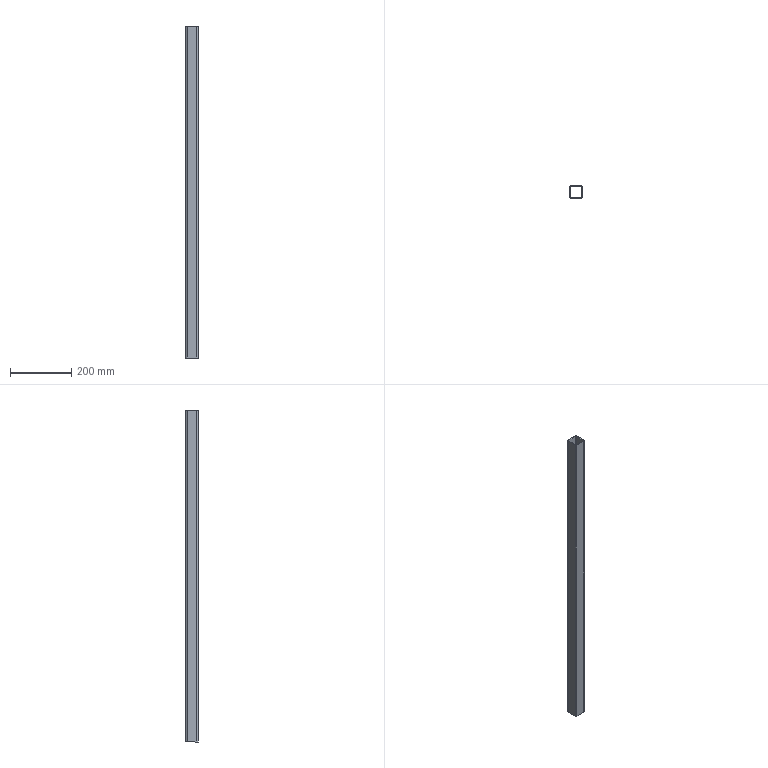Part | SolidWorks | features Fillet 2, Extrusion 1 | 1 solid | 18 faces | box 40 x 40 x 1082 mm | volume 317782 mm3 | plane 10 | cylinder 8 | commonest cylinder face diameters 4 x4 8 x4
STEP:
#1=CARTESIAN_POINT('',(20.,-16.,1082.));
#2=VERTEX_POINT('',#1);
#3=CARTESIAN_POINT('',(20.,16.,1082.));
#4=VERTEX_POINT('',#3);
#5=CARTESIAN_POINT('',(20.,20.,1082.));
#6=DIRECTION('',(0.,1.,0.));
#7=VECTOR('',#6,1000.);
#8=LINE('',#5,#7);
#9=EDGE_CURVE('',#2,#4,#8,.T.);
#10=ORIENTED_EDGE('',*,*,#9,.T.);
#11=CARTESIAN_POINT('',(16.,20.,1082.));
#12=VERTEX_POINT('',#11);
#13=CARTESIAN_POINT('',(16.,16.,1082.));
#14=DIRECTION('',(0.,0.,1.));
#15=DIRECTION('',(1.,0.,0.));
#16=AXIS2_PLACEMENT_3D('',#13,#14,#15);
#17=CIRCLE('',#16,4.);
#18=EDGE_CURVE('',#4,#12,#17,.T.);
#19=ORIENTED_EDGE('',*,*,#18,.T.);
#20=CARTESIAN_POINT('',(-16.,20.,1082.));
#21=VERTEX_POINT('',#20);
#22=CARTESIAN_POINT('',(-20.,20.,1082.));
#23=DIRECTION('',(-1.,0.,0.));
#24=VECTOR('',#23,1000.);
#25=LINE('',#22,#24);
#26=EDGE_CURVE('',#12,#21,#25,.T.);
#27=ORIENTED_EDGE('',*,*,#26,.T.);
#28=CARTESIAN_POINT('',(-20.,16.,1082.));
#29=VERTEX_POINT('',#28);
#30=CARTESIAN_POINT('',(-16.,16.,1082.));
#31=DIRECTION('',(0.,0.,1.));
#32=DIRECTION('',(1.,0.,0.));
#33=AXIS2_PLACEMENT_3D('',#30,#31,#32);
#34=CIRCLE('',#33,4.);
#35=EDGE_CURVE('',#21,#29,#34,.T.);
#36=ORIENTED_EDGE('',*,*,#35,.T.);
#37=CARTESIAN_POINT('',(-20.,-16.,1082.));
#38=VERTEX_POINT('',#37);
#39=CARTESIAN_POINT('',(-20.,20.,1082.));
#40=DIRECTION('',(0.,-1.,0.));
#41=VECTOR('',#40,1000.);
#42=LINE('',#39,#41);
#43=EDGE_CURVE('',#29,#38,#42,.T.);
#44=ORIENTED_EDGE('',*,*,#43,.T.);
#45=CARTESIAN_POINT('',(-16.,-20.,1082.));
#46=VERTEX_POINT('',#45);
#47=CARTESIAN_POINT('',(-16.,-16.,1082.));
#48=DIRECTION('',(0.,0.,1.));
#49=DIRECTION('',(1.,0.,0.));
#50=AXIS2_PLACEMENT_3D('',#47,#48,#49);
#51=CIRCLE('',#50,4.);
#52=EDGE_CURVE('',#38,#46,#51,.T.);
#53=ORIENTED_EDGE('',*,*,#52,.T.);
#54=CARTESIAN_POINT('',(16.,-20.,1082.));
#55=VERTEX_POINT('',#54);
#56=CARTESIAN_POINT('',(-20.,-20.,1082.));
#57=DIRECTION('',(1.,0.,0.));
#58=VECTOR('',#57,1000.);
#59=LINE('',#56,#58);
#60=EDGE_CURVE('',#46,#55,#59,.T.);
#61=ORIENTED_EDGE('',*,*,#60,.T.);
#62=CARTESIAN_POINT('',(16.,-16.,1082.));
#63=DIRECTION('',(0.,0.,1.));
#64=DIRECTION('',(1.,0.,0.));
#65=AXIS2_PLACEMENT_3D('',#62,#63,#64);
#66=CIRCLE('',#65,4.);
#67=EDGE_CURVE('',#55,#2,#66,.T.);
#68=ORIENTED_EDGE('',*,*,#67,.T.);
#69=EDGE_LOOP('',(#10,#19,#27,#36,#44,#53,#61,#68));
#70=FACE_OUTER_BOUND('',#69,.T.);
#71=CARTESIAN_POINT('',(16.,18.,1082.));
#72=VERTEX_POINT('',#71);
#73=CARTESIAN_POINT('',(-16.,18.,1082.));
#74=VERTEX_POINT('',#73);
#75=CARTESIAN_POINT('',(-18.,18.,1082.));
#76=DIRECTION('',(-1.,0.,0.));
#77=VECTOR('',#76,1000.);
#78=LINE('',#75,#77);
#79=EDGE_CURVE('',#72,#74,#78,.T.);
#80=ORIENTED_EDGE('',*,*,#79,.F.);
#81=CARTESIAN_POINT('',(18.,16.,1082.));
#82=VERTEX_POINT('',#81);
#83=CARTESIAN_POINT('',(16.,16.,1082.));
#84=DIRECTION('',(0.,0.,-1.));
#85=DIRECTION('',(1.,0.,0.));
#86=AXIS2_PLACEMENT_3D('',#83,#84,#85);
#87=CIRCLE('',#86,2.);
#88=EDGE_CURVE('',#72,#82,#87,.T.);
#89=ORIENTED_EDGE('',*,*,#88,.T.);
#90=CARTESIAN_POINT('',(18.,-16.,1082.));
#91=VERTEX_POINT('',#90);
#92=CARTESIAN_POINT('',(18.,18.,1082.));
#93=DIRECTION('',(0.,1.,0.));
#94=VECTOR('',#93,1000.);
#95=LINE('',#92,#94);
#96=EDGE_CURVE('',#91,#82,#95,.T.);
#97=ORIENTED_EDGE('',*,*,#96,.F.);
#98=CARTESIAN_POINT('',(16.,-18.,1082.));
#99=VERTEX_POINT('',#98);
#100=CARTESIAN_POINT('',(16.,-16.,1082.));
#101=DIRECTION('',(0.,0.,-1.));
#102=DIRECTION('',(1.,0.,0.));
#103=AXIS2_PLACEMENT_3D('',#100,#101,#102);
#104=CIRCLE('',#103,2.);
#105=EDGE_CURVE('',#91,#99,#104,.T.);
#106=ORIENTED_EDGE('',*,*,#105,.T.);
#107=CARTESIAN_POINT('',(-16.,-18.,1082.));
#108=VERTEX_POINT('',#107);
#109=CARTESIAN_POINT('',(-18.,-18.,1082.));
#110=DIRECTION('',(1.,0.,0.));
#111=VECTOR('',#110,1000.);
#112=LINE('',#109,#111);
#113=EDGE_CURVE('',#108,#99,#112,.T.);
#114=ORIENTED_EDGE('',*,*,#113,.F.);
#115=CARTESIAN_POINT('',(-18.,-16.,1082.));
#116=VERTEX_POINT('',#115);
#117=CARTESIAN_POINT('',(-16.,-16.,1082.));
#118=DIRECTION('',(0.,0.,-1.));
#119=DIRECTION('',(1.,0.,0.));
#120=AXIS2_PLACEMENT_3D('',#117,#118,#119);
#121=CIRCLE('',#120,2.);
#122=EDGE_CURVE('',#108,#116,#121,.T.);
#123=ORIENTED_EDGE('',*,*,#122,.T.);
#124=CARTESIAN_POINT('',(-18.,16.,1082.));
#125=VERTEX_POINT('',#124);
#126=CARTESIAN_POINT('',(-18.,18.,1082.));
#127=DIRECTION('',(0.,-1.,0.));
#128=VECTOR('',#127,1000.);
#129=LINE('',#126,#128);
#130=EDGE_CURVE('',#125,#116,#129,.T.);
#131=ORIENTED_EDGE('',*,*,#130,.F.);
#132=CARTESIAN_POINT('',(-16.,16.,1082.));
#133=DIRECTION('',(0.,0.,-1.));
#134=DIRECTION('',(1.,0.,0.));
#135=AXIS2_PLACEMENT_3D('',#132,#133,#134);
#136=CIRCLE('',#135,2.);
#137=EDGE_CURVE('',#125,#74,#136,.T.);
#138=ORIENTED_EDGE('',*,*,#137,.T.);
#139=EDGE_LOOP('',(#80,#89,#97,#106,#114,#123,#131,#138));
#140=FACE_BOUND('',#139,.T.);
#141=CARTESIAN_POINT('',(0.,0.,1082.));
#142=DIRECTION('',(0.,0.,1.));
#143=DIRECTION('',(1.,0.,0.));
#144=AXIS2_PLACEMENT_3D('',#141,#142,#143);
#145=PLANE('',#144);
#146=ADVANCED_FACE('',(#70,#140),#145,.T.);
#147=CARTESIAN_POINT('',(16.,20.,0.));
#148=VERTEX_POINT('',#147);
#149=CARTESIAN_POINT('',(-16.,20.,0.));
#150=VERTEX_POINT('',#149);
#151=CARTESIAN_POINT('',(-20.,20.,0.));
#152=DIRECTION('',(-1.,0.,0.));
#153=VECTOR('',#152,1000.);
#154=LINE('',#151,#153);
#155=EDGE_CURVE('',#148,#150,#154,.T.);
#156=ORIENTED_EDGE('',*,*,#155,.F.);
#157=CARTESIAN_POINT('',(20.,16.,0.));
#158=VERTEX_POINT('',#157);
#159=CARTESIAN_POINT('',(16.,16.,0.));
#160=DIRECTION('',(0.,0.,-1.));
#161=DIRECTION('',(1.,0.,0.));
#162=AXIS2_PLACEMENT_3D('',#159,#160,#161);
#163=CIRCLE('',#162,4.);
#164=EDGE_CURVE('',#148,#158,#163,.T.);
#165=ORIENTED_EDGE('',*,*,#164,.T.);
#166=CARTESIAN_POINT('',(20.,-16.,0.));
#167=VERTEX_POINT('',#166);
#168=CARTESIAN_POINT('',(20.,20.,0.));
#169=DIRECTION('',(0.,1.,0.));
#170=VECTOR('',#169,1000.);
#171=LINE('',#168,#170);
#172=EDGE_CURVE('',#167,#158,#171,.T.);
#173=ORIENTED_EDGE('',*,*,#172,.F.);
#174=CARTESIAN_POINT('',(16.,-20.,0.));
#175=VERTEX_POINT('',#174);
#176=CARTESIAN_POINT('',(16.,-16.,0.));
#177=DIRECTION('',(0.,0.,-1.));
#178=DIRECTION('',(1.,0.,0.));
#179=AXIS2_PLACEMENT_3D('',#176,#177,#178);
#180=CIRCLE('',#179,4.);
#181=EDGE_CURVE('',#167,#175,#180,.T.);
#182=ORIENTED_EDGE('',*,*,#181,.T.);
#183=CARTESIAN_POINT('',(-16.,-20.,0.));
#184=VERTEX_POINT('',#183);
#185=CARTESIAN_POINT('',(-20.,-20.,0.));
#186=DIRECTION('',(1.,0.,0.));
#187=VECTOR('',#186,1000.);
#188=LINE('',#185,#187);
#189=EDGE_CURVE('',#184,#175,#188,.T.);
#190=ORIENTED_EDGE('',*,*,#189,.F.);
#191=CARTESIAN_POINT('',(-20.,-16.,0.));
#192=VERTEX_POINT('',#191);
#193=CARTESIAN_POINT('',(-16.,-16.,0.));
#194=DIRECTION('',(0.,0.,-1.));
#195=DIRECTION('',(1.,0.,0.));
#196=AXIS2_PLACEMENT_3D('',#193,#194,#195);
#197=CIRCLE('',#196,4.);
#198=EDGE_CURVE('',#184,#192,#197,.T.);
#199=ORIENTED_EDGE('',*,*,#198,.T.);
#200=CARTESIAN_POINT('',(-20.,16.,0.));
#201=VERTEX_POINT('',#200);
#202=CARTESIAN_POINT('',(-20.,20.,0.));
#203=DIRECTION('',(0.,-1.,0.));
#204=VECTOR('',#203,1000.);
#205=LINE('',#202,#204);
#206=EDGE_CURVE('',#201,#192,#205,.T.);
#207=ORIENTED_EDGE('',*,*,#206,.F.);
#208=CARTESIAN_POINT('',(-16.,16.,0.));
#209=DIRECTION('',(0.,0.,-1.));
#210=DIRECTION('',(1.,0.,0.));
#211=AXIS2_PLACEMENT_3D('',#208,#209,#210);
#212=CIRCLE('',#211,4.);
#213=EDGE_CURVE('',#201,#150,#212,.T.);
#214=ORIENTED_EDGE('',*,*,#213,.T.);
#215=EDGE_LOOP('',(#156,#165,#173,#182,#190,#199,#207,#214));
#216=FACE_OUTER_BOUND('',#215,.T.);
#217=CARTESIAN_POINT('',(-16.,-18.,0.));
#218=VERTEX_POINT('',#217);
#219=CARTESIAN_POINT('',(16.,-18.,0.));
#220=VERTEX_POINT('',#219);
#221=CARTESIAN_POINT('',(-18.,-18.,0.));
#222=DIRECTION('',(1.,0.,0.));
#223=VECTOR('',#222,1000.);
#224=LINE('',#221,#223);
#225=EDGE_CURVE('',#218,#220,#224,.T.);
#226=ORIENTED_EDGE('',*,*,#225,.T.);
#227=CARTESIAN_POINT('',(18.,-16.,0.));
#228=VERTEX_POINT('',#227);
#229=CARTESIAN_POINT('',(16.,-16.,0.));
#230=DIRECTION('',(0.,0.,1.));
#231=DIRECTION('',(1.,0.,0.));
#232=AXIS2_PLACEMENT_3D('',#229,#230,#231);
#233=CIRCLE('',#232,2.);
#234=EDGE_CURVE('',#220,#228,#233,.T.);
#235=ORIENTED_EDGE('',*,*,#234,.T.);
#236=CARTESIAN_POINT('',(18.,16.,0.));
#237=VERTEX_POINT('',#236);
#238=CARTESIAN_POINT('',(18.,18.,0.));
#239=DIRECTION('',(0.,1.,0.));
#240=VECTOR('',#239,1000.);
#241=LINE('',#238,#240);
#242=EDGE_CURVE('',#228,#237,#241,.T.);
#243=ORIENTED_EDGE('',*,*,#242,.T.);
#244=CARTESIAN_POINT('',(16.,18.,0.));
#245=VERTEX_POINT('',#244);
#246=CARTESIAN_POINT('',(16.,16.,0.));
#247=DIRECTION('',(0.,0.,1.));
#248=DIRECTION('',(1.,0.,0.));
#249=AXIS2_PLACEMENT_3D('',#246,#247,#248);
#250=CIRCLE('',#249,2.);
#251=EDGE_CURVE('',#237,#245,#250,.T.);
#252=ORIENTED_EDGE('',*,*,#251,.T.);
#253=CARTESIAN_POINT('',(-16.,18.,0.));
#254=VERTEX_POINT('',#253);
#255=CARTESIAN_POINT('',(-18.,18.,0.));
#256=DIRECTION('',(-1.,0.,0.));
#257=VECTOR('',#256,1000.);
#258=LINE('',#255,#257);
#259=EDGE_CURVE('',#245,#254,#258,.T.);
#260=ORIENTED_EDGE('',*,*,#259,.T.);
#261=CARTESIAN_POINT('',(-18.,16.,0.));
#262=VERTEX_POINT('',#261);
#263=CARTESIAN_POINT('',(-16.,16.,0.));
#264=DIRECTION('',(0.,0.,1.));
#265=DIRECTION('',(1.,0.,0.));
#266=AXIS2_PLACEMENT_3D('',#263,#264,#265);
#267=CIRCLE('',#266,2.);
#268=EDGE_CURVE('',#254,#262,#267,.T.);
#269=ORIENTED_EDGE('',*,*,#268,.T.);
#270=CARTESIAN_POINT('',(-18.,-16.,0.));
#271=VERTEX_POINT('',#270);
#272=CARTESIAN_POINT('',(-18.,18.,0.));
#273=DIRECTION('',(0.,-1.,0.));
#274=VECTOR('',#273,1000.);
#275=LINE('',#272,#274);
#276=EDGE_CURVE('',#262,#271,#275,.T.);
#277=ORIENTED_EDGE('',*,*,#276,.T.);
#278=CARTESIAN_POINT('',(-16.,-16.,0.));
#279=DIRECTION('',(0.,0.,1.));
#280=DIRECTION('',(1.,0.,0.));
#281=AXIS2_PLACEMENT_3D('',#278,#279,#280);
#282=CIRCLE('',#281,2.);
#283=EDGE_CURVE('',#271,#218,#282,.T.);
#284=ORIENTED_EDGE('',*,*,#283,.T.);
#285=EDGE_LOOP('',(#226,#235,#243,#252,#260,#269,#277,#284));
#286=FACE_BOUND('',#285,.T.);
#287=CARTESIAN_POINT('',(0.,0.,0.));
#288=DIRECTION('',(0.,0.,1.));
#289=DIRECTION('',(1.,0.,0.));
#290=AXIS2_PLACEMENT_3D('',#287,#288,#289);
#291=PLANE('',#290);
#292=ADVANCED_FACE('',(#216,#286),#291,.F.);
#293=ORIENTED_EDGE('',*,*,#172,.T.);
#294=CARTESIAN_POINT('',(20.,16.,1082.));
#295=DIRECTION('',(0.,0.,1.));
#296=VECTOR('',#295,1000.);
#297=LINE('',#294,#296);
#298=EDGE_CURVE('',#158,#4,#297,.T.);
#299=ORIENTED_EDGE('',*,*,#298,.T.);
#300=ORIENTED_EDGE('',*,*,#9,.F.);
#301=CARTESIAN_POINT('',(20.,-16.,1082.));
#302=DIRECTION('',(0.,0.,-1.));
#303=VECTOR('',#302,1000.);
#304=LINE('',#301,#303);
#305=EDGE_CURVE('',#2,#167,#304,.T.);
#306=ORIENTED_EDGE('',*,*,#305,.T.);
#307=EDGE_LOOP('',(#293,#299,#300,#306));
#308=FACE_OUTER_BOUND('',#307,.T.);
#309=CARTESIAN_POINT('',(20.,20.,1082.));
#310=DIRECTION('',(-1.,0.,0.));
#311=DIRECTION('',(0.,0.,1.));
#312=AXIS2_PLACEMENT_3D('',#309,#310,#311);
#313=PLANE('',#312);
#314=ADVANCED_FACE('',(#308),#313,.F.);
#315=ORIENTED_EDGE('',*,*,#26,.F.);
#316=CARTESIAN_POINT('',(16.,20.,1082.));
#317=DIRECTION('',(0.,0.,-1.));
#318=VECTOR('',#317,1000.);
#319=LINE('',#316,#318);
#320=EDGE_CURVE('',#12,#148,#319,.T.);
#321=ORIENTED_EDGE('',*,*,#320,.T.);
#322=ORIENTED_EDGE('',*,*,#155,.T.);
#323=CARTESIAN_POINT('',(-16.,20.,1082.));
#324=DIRECTION('',(0.,0.,1.));
#325=VECTOR('',#324,1000.);
#326=LINE('',#323,#325);
#327=EDGE_CURVE('',#150,#21,#326,.T.);
#328=ORIENTED_EDGE('',*,*,#327,.T.);
#329=EDGE_LOOP('',(#315,#321,#322,#328));
#330=FACE_OUTER_BOUND('',#329,.T.);
#331=CARTESIAN_POINT('',(-20.,20.,1082.));
#332=DIRECTION('',(0.,-1.,0.));
#333=DIRECTION('',(0.,0.,-1.));
#334=AXIS2_PLACEMENT_3D('',#331,#332,#333);
#335=PLANE('',#334);
#336=ADVANCED_FACE('',(#330),#335,.F.);
#337=ORIENTED_EDGE('',*,*,#43,.F.);
#338=CARTESIAN_POINT('',(-20.,16.,1082.));
#339=DIRECTION('',(0.,0.,-1.));
#340=VECTOR('',#339,1000.);
#341=LINE('',#338,#340);
#342=EDGE_CURVE('',#29,#201,#341,.T.);
#343=ORIENTED_EDGE('',*,*,#342,.T.);
#344=ORIENTED_EDGE('',*,*,#206,.T.);
#345=CARTESIAN_POINT('',(-20.,-16.,1082.));
#346=DIRECTION('',(0.,0.,1.));
#347=VECTOR('',#346,1000.);
#348=LINE('',#345,#347);
#349=EDGE_CURVE('',#192,#38,#348,.T.);
#350=ORIENTED_EDGE('',*,*,#349,.T.);
#351=EDGE_LOOP('',(#337,#343,#344,#350));
#352=FACE_OUTER_BOUND('',#351,.T.);
#353=CARTESIAN_POINT('',(-20.,20.,1082.));
#354=DIRECTION('',(1.,0.,0.));
#355=DIRECTION('',(0.,0.,-1.));
#356=AXIS2_PLACEMENT_3D('',#353,#354,#355);
#357=PLANE('',#356);
#358=ADVANCED_FACE('',(#352),#357,.F.);
#359=ORIENTED_EDGE('',*,*,#189,.T.);
#360=CARTESIAN_POINT('',(16.,-20.,1082.));
#361=DIRECTION('',(0.,0.,1.));
#362=VECTOR('',#361,1000.);
#363=LINE('',#360,#362);
#364=EDGE_CURVE('',#175,#55,#363,.T.);
#365=ORIENTED_EDGE('',*,*,#364,.T.);
#366=ORIENTED_EDGE('',*,*,#60,.F.);
#367=CARTESIAN_POINT('',(-16.,-20.,1082.));
#368=DIRECTION('',(0.,0.,-1.));
#369=VECTOR('',#368,1000.);
#370=LINE('',#367,#369);
#371=EDGE_CURVE('',#46,#184,#370,.T.);
#372=ORIENTED_EDGE('',*,*,#371,.T.);
#373=EDGE_LOOP('',(#359,#365,#366,#372));
#374=FACE_OUTER_BOUND('',#373,.T.);
#375=CARTESIAN_POINT('',(-20.,-20.,1082.));
#376=DIRECTION('',(0.,1.,0.));
#377=DIRECTION('',(0.,0.,1.));
#378=AXIS2_PLACEMENT_3D('',#375,#376,#377);
#379=PLANE('',#378);
#380=ADVANCED_FACE('',(#374),#379,.F.);
#381=ORIENTED_EDGE('',*,*,#96,.T.);
#382=CARTESIAN_POINT('',(18.,16.,0.));
#383=DIRECTION('',(0.,0.,-1.));
#384=VECTOR('',#383,1000.);
#385=LINE('',#382,#384);
#386=EDGE_CURVE('',#82,#237,#385,.T.);
#387=ORIENTED_EDGE('',*,*,#386,.T.);
#388=ORIENTED_EDGE('',*,*,#242,.F.);
#389=CARTESIAN_POINT('',(18.,-16.,1082.));
#390=DIRECTION('',(0.,0.,1.));
#391=VECTOR('',#390,1000.);
#392=LINE('',#389,#391);
#393=EDGE_CURVE('',#228,#91,#392,.T.);
#394=ORIENTED_EDGE('',*,*,#393,.T.);
#395=EDGE_LOOP('',(#381,#387,#388,#394));
#396=FACE_OUTER_BOUND('',#395,.T.);
#397=CARTESIAN_POINT('',(18.,18.,1082.));
#398=DIRECTION('',(-1.,0.,0.));
#399=DIRECTION('',(0.,0.,1.));
#400=AXIS2_PLACEMENT_3D('',#397,#398,#399);
#401=PLANE('',#400);
#402=ADVANCED_FACE('',(#396),#401,.T.);
#403=ORIENTED_EDGE('',*,*,#259,.F.);
#404=CARTESIAN_POINT('',(16.,18.,1082.));
#405=DIRECTION('',(0.,0.,1.));
#406=VECTOR('',#405,1000.);
#407=LINE('',#404,#406);
#408=EDGE_CURVE('',#245,#72,#407,.T.);
#409=ORIENTED_EDGE('',*,*,#408,.T.);
#410=ORIENTED_EDGE('',*,*,#79,.T.);
#411=CARTESIAN_POINT('',(-16.,18.,0.));
#412=DIRECTION('',(0.,0.,-1.));
#413=VECTOR('',#412,1000.);
#414=LINE('',#411,#413);
#415=EDGE_CURVE('',#74,#254,#414,.T.);
#416=ORIENTED_EDGE('',*,*,#415,.T.);
#417=EDGE_LOOP('',(#403,#409,#410,#416));
#418=FACE_OUTER_BOUND('',#417,.T.);
#419=CARTESIAN_POINT('',(-18.,18.,1082.));
#420=DIRECTION('',(0.,-1.,0.));
#421=DIRECTION('',(0.,0.,-1.));
#422=AXIS2_PLACEMENT_3D('',#419,#420,#421);
#423=PLANE('',#422);
#424=ADVANCED_FACE('',(#418),#423,.T.);
#425=ORIENTED_EDGE('',*,*,#276,.F.);
#426=CARTESIAN_POINT('',(-18.,16.,1082.));
#427=DIRECTION('',(0.,0.,1.));
#428=VECTOR('',#427,1000.);
#429=LINE('',#426,#428);
#430=EDGE_CURVE('',#262,#125,#429,.T.);
#431=ORIENTED_EDGE('',*,*,#430,.T.);
#432=ORIENTED_EDGE('',*,*,#130,.T.);
#433=CARTESIAN_POINT('',(-18.,-16.,0.));
#434=DIRECTION('',(0.,0.,-1.));
#435=VECTOR('',#434,1000.);
#436=LINE('',#433,#435);
#437=EDGE_CURVE('',#116,#271,#436,.T.);
#438=ORIENTED_EDGE('',*,*,#437,.T.);
#439=EDGE_LOOP('',(#425,#431,#432,#438));
#440=FACE_OUTER_BOUND('',#439,.T.);
#441=CARTESIAN_POINT('',(-18.,18.,1082.));
#442=DIRECTION('',(1.,0.,0.));
#443=DIRECTION('',(0.,0.,-1.));
#444=AXIS2_PLACEMENT_3D('',#441,#442,#443);
#445=PLANE('',#444);
#446=ADVANCED_FACE('',(#440),#445,.T.);
#447=ORIENTED_EDGE('',*,*,#225,.F.);
#448=CARTESIAN_POINT('',(-16.,-18.,1082.));
#449=DIRECTION('',(0.,0.,1.));
#450=VECTOR('',#449,1000.);
#451=LINE('',#448,#450);
#452=EDGE_CURVE('',#218,#108,#451,.T.);
#453=ORIENTED_EDGE('',*,*,#452,.T.);
#454=ORIENTED_EDGE('',*,*,#113,.T.);
#455=CARTESIAN_POINT('',(16.,-18.,0.));
#456=DIRECTION('',(0.,0.,-1.));
#457=VECTOR('',#456,1000.);
#458=LINE('',#455,#457);
#459=EDGE_CURVE('',#99,#220,#458,.T.);
#460=ORIENTED_EDGE('',*,*,#459,.T.);
#461=EDGE_LOOP('',(#447,#453,#454,#460));
#462=FACE_OUTER_BOUND('',#461,.T.);
#463=CARTESIAN_POINT('',(-18.,-18.,1082.));
#464=DIRECTION('',(0.,1.,0.));
#465=DIRECTION('',(0.,0.,1.));
#466=AXIS2_PLACEMENT_3D('',#463,#464,#465);
#467=PLANE('',#466);
#468=ADVANCED_FACE('',(#462),#467,.T.);
#469=ORIENTED_EDGE('',*,*,#88,.F.);
#470=ORIENTED_EDGE('',*,*,#408,.F.);
#471=ORIENTED_EDGE('',*,*,#251,.F.);
#472=ORIENTED_EDGE('',*,*,#386,.F.);
#473=EDGE_LOOP('',(#469,#470,#471,#472));
#474=FACE_OUTER_BOUND('',#473,.T.);
#475=CARTESIAN_POINT('',(16.,16.,1082.));
#476=DIRECTION('',(0.,0.,1.));
#477=DIRECTION('',(1.,0.,0.));
#478=AXIS2_PLACEMENT_3D('',#475,#476,#477);
#479=CYLINDRICAL_SURFACE('',#478,2.);
#480=ADVANCED_FACE('',(#474),#479,.F.);
#481=ORIENTED_EDGE('',*,*,#137,.F.);
#482=ORIENTED_EDGE('',*,*,#430,.F.);
#483=ORIENTED_EDGE('',*,*,#268,.F.);
#484=ORIENTED_EDGE('',*,*,#415,.F.);
#485=EDGE_LOOP('',(#481,#482,#483,#484));
#486=FACE_OUTER_BOUND('',#485,.T.);
#487=CARTESIAN_POINT('',(-16.,16.,1082.));
#488=DIRECTION('',(0.,0.,1.));
#489=DIRECTION('',(1.,0.,0.));
#490=AXIS2_PLACEMENT_3D('',#487,#488,#489);
#491=CYLINDRICAL_SURFACE('',#490,2.);
#492=ADVANCED_FACE('',(#486),#491,.F.);
#493=ORIENTED_EDGE('',*,*,#122,.F.);
#494=ORIENTED_EDGE('',*,*,#452,.F.);
#495=ORIENTED_EDGE('',*,*,#283,.F.);
#496=ORIENTED_EDGE('',*,*,#437,.F.);
#497=EDGE_LOOP('',(#493,#494,#495,#496));
#498=FACE_OUTER_BOUND('',#497,.T.);
#499=CARTESIAN_POINT('',(-16.,-16.,1082.));
#500=DIRECTION('',(0.,0.,1.));
#501=DIRECTION('',(1.,0.,0.));
#502=AXIS2_PLACEMENT_3D('',#499,#500,#501);
#503=CYLINDRICAL_SURFACE('',#502,2.);
#504=ADVANCED_FACE('',(#498),#503,.F.);
#505=ORIENTED_EDGE('',*,*,#105,.F.);
#506=ORIENTED_EDGE('',*,*,#393,.F.);
#507=ORIENTED_EDGE('',*,*,#234,.F.);
#508=ORIENTED_EDGE('',*,*,#459,.F.);
#509=EDGE_LOOP('',(#505,#506,#507,#508));
#510=FACE_OUTER_BOUND('',#509,.T.);
#511=CARTESIAN_POINT('',(16.,-16.,1082.));
#512=DIRECTION('',(0.,0.,1.));
#513=DIRECTION('',(1.,0.,0.));
#514=AXIS2_PLACEMENT_3D('',#511,#512,#513);
#515=CYLINDRICAL_SURFACE('',#514,2.);
#516=ADVANCED_FACE('',(#510),#515,.F.);
#517=ORIENTED_EDGE('',*,*,#18,.F.);
#518=ORIENTED_EDGE('',*,*,#298,.F.);
#519=ORIENTED_EDGE('',*,*,#164,.F.);
#520=ORIENTED_EDGE('',*,*,#320,.F.);
#521=EDGE_LOOP('',(#517,#518,#519,#520));
#522=FACE_OUTER_BOUND('',#521,.T.);
#523=CARTESIAN_POINT('',(16.,16.,1082.));
#524=DIRECTION('',(0.,0.,-1.));
#525=DIRECTION('',(-1.,0.,0.));
#526=AXIS2_PLACEMENT_3D('',#523,#524,#525);
#527=CYLINDRICAL_SURFACE('',#526,4.);
#528=ADVANCED_FACE('',(#522),#527,.T.);
#529=ORIENTED_EDGE('',*,*,#67,.F.);
#530=ORIENTED_EDGE('',*,*,#364,.F.);
#531=ORIENTED_EDGE('',*,*,#181,.F.);
#532=ORIENTED_EDGE('',*,*,#305,.F.);
#533=EDGE_LOOP('',(#529,#530,#531,#532));
#534=FACE_OUTER_BOUND('',#533,.T.);
#535=CARTESIAN_POINT('',(16.,-16.,1082.));
#536=DIRECTION('',(0.,0.,-1.));
#537=DIRECTION('',(-1.,0.,0.));
#538=AXIS2_PLACEMENT_3D('',#535,#536,#537);
#539=CYLINDRICAL_SURFACE('',#538,4.);
#540=ADVANCED_FACE('',(#534),#539,.T.);
#541=ORIENTED_EDGE('',*,*,#35,.F.);
#542=ORIENTED_EDGE('',*,*,#327,.F.);
#543=ORIENTED_EDGE('',*,*,#213,.F.);
#544=ORIENTED_EDGE('',*,*,#342,.F.);
#545=EDGE_LOOP('',(#541,#542,#543,#544));
#546=FACE_OUTER_BOUND('',#545,.T.);
#547=CARTESIAN_POINT('',(-16.,16.,1082.));
#548=DIRECTION('',(0.,0.,-1.));
#549=DIRECTION('',(-1.,0.,0.));
#550=AXIS2_PLACEMENT_3D('',#547,#548,#549);
#551=CYLINDRICAL_SURFACE('',#550,4.);
#552=ADVANCED_FACE('',(#546),#551,.T.);
#553=ORIENTED_EDGE('',*,*,#52,.F.);
#554=ORIENTED_EDGE('',*,*,#349,.F.);
#555=ORIENTED_EDGE('',*,*,#198,.F.);
#556=ORIENTED_EDGE('',*,*,#371,.F.);
#557=EDGE_LOOP('',(#553,#554,#555,#556));
#558=FACE_OUTER_BOUND('',#557,.T.);
#559=CARTESIAN_POINT('',(-16.,-16.,1082.));
#560=DIRECTION('',(0.,0.,-1.));
#561=DIRECTION('',(-1.,0.,0.));
#562=AXIS2_PLACEMENT_3D('',#559,#560,#561);
#563=CYLINDRICAL_SURFACE('',#562,4.);
#564=ADVANCED_FACE('',(#558),#563,.T.);
#565=CLOSED_SHELL('',(#146,#292,#314,#336,#358,#380,#402,#424,#446,#468,#480,#492,#504,#516,#528,#540,#552,#564));
#566=MANIFOLD_SOLID_BREP('',#565);
#567=CARTESIAN_POINT('',(0.,0.,0.));
#568=DIRECTION('',(0.,0.,1.));
#569=DIRECTION('',(1.,0.,0.));
#570=AXIS2_PLACEMENT_3D('',#567,#568,#569);
#571=(LENGTH_UNIT()NAMED_UNIT(*)SI_UNIT(.MILLI.,.METRE.));
#572=UNCERTAINTY_MEASURE_WITH_UNIT(LENGTH_MEASURE(0.00001),#571,'','');
#573=(NAMED_UNIT(*)PLANE_ANGLE_UNIT()SI_UNIT($,.RADIAN.));
#574=(NAMED_UNIT(*)SI_UNIT($,.STERADIAN.)SOLID_ANGLE_UNIT());
#575=(GEOMETRIC_REPRESENTATION_CONTEXT(3)GLOBAL_UNCERTAINTY_ASSIGNED_CONTEXT((#572))GLOBAL_UNIT_ASSIGNED_CONTEXT((#571,#573,#574))REPRESENTATION_CONTEXT('',''));
#576=ADVANCED_BREP_SHAPE_REPRESENTATION('',(#566,#570),#575);